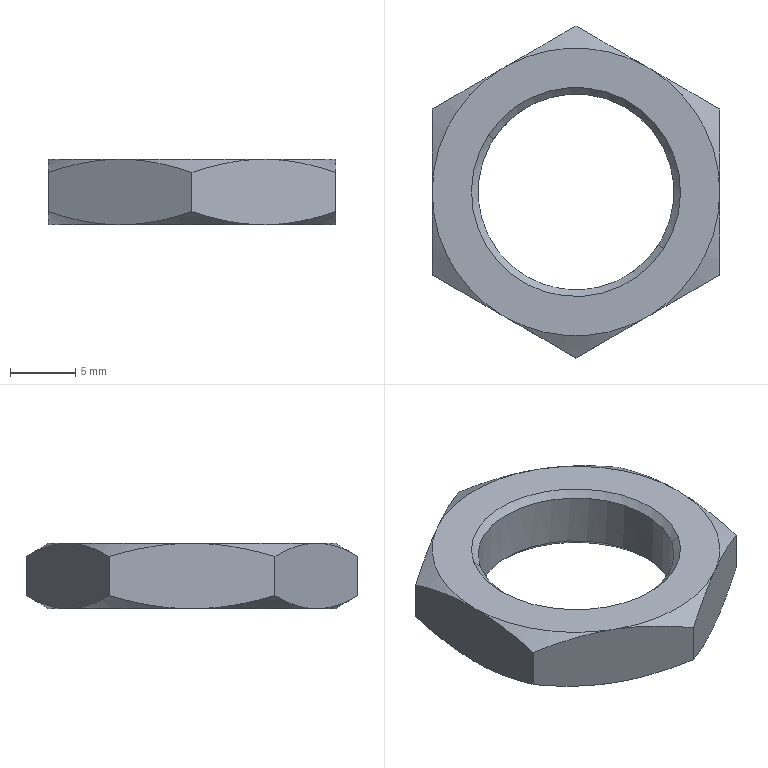Part | STEP file | Nut.1.stp | 1 solid | 28 faces | box 22 x 25.403 x 5 mm | volume 1177 mm3 | cone 18 | plane 8 | cylinder 2 | commonest cylinder face diameters 15 x2